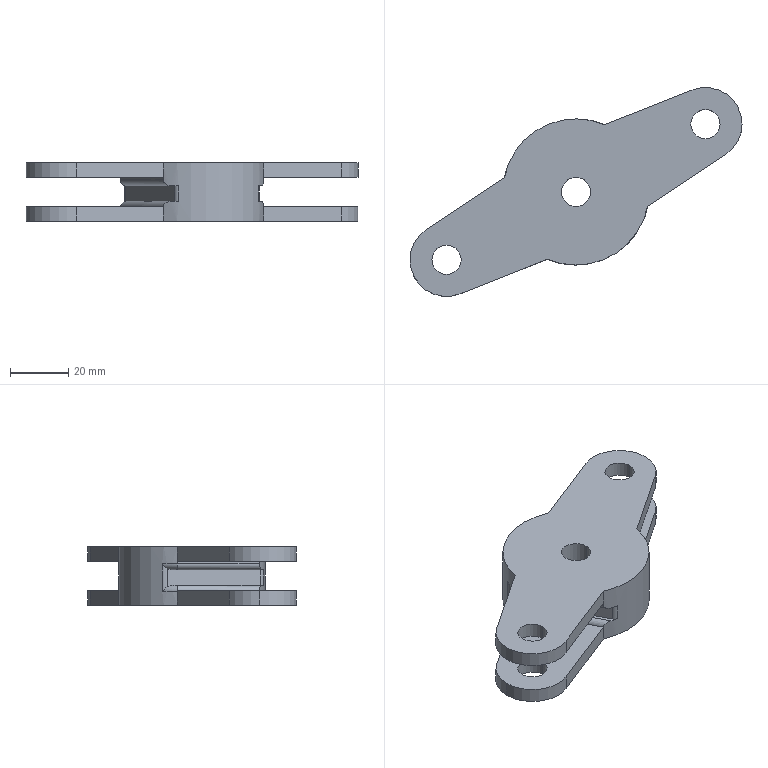Part | SolidWorks | features ICE 3, Fillet 2, Extrusion 1 | 1 solid | 52 faces | box 113.562 x 71.441 x 20 mm | volume 52250 mm3 | cylinder 27 | plane 22 | torus 3 | commonest cylinder face diameters 10 x10 4 x9 25 x6 50 x2